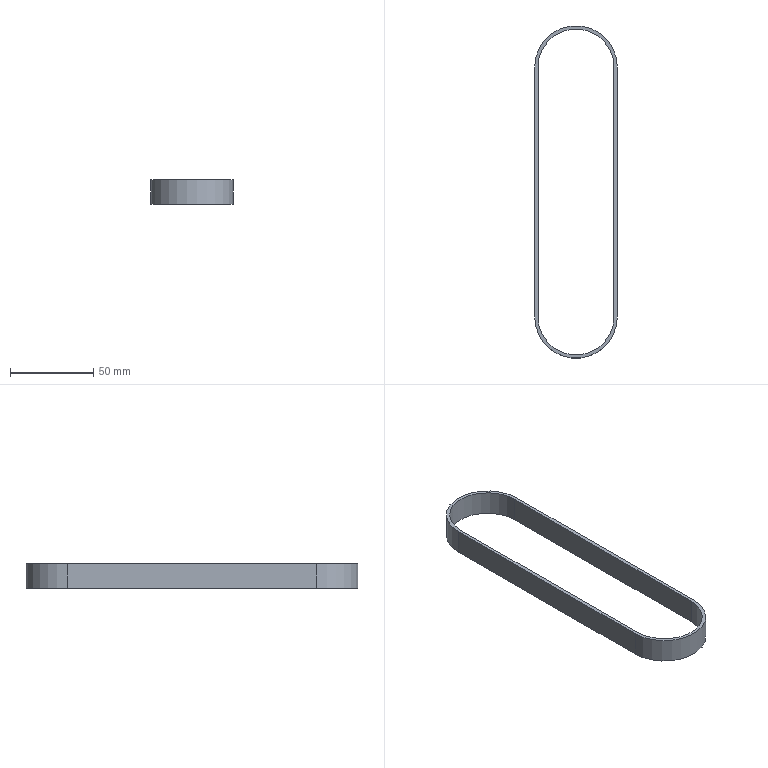Part | STEP file | Belt 1-1^ND25021-刻码机 | 1 solid | 10 faces | box 49.6 x 199.6 x 15 mm | volume 13486 mm3 | plane 6 | cylinder 4 | commonest cylinder face diameters 45.6 x2 49.6 x2
STEP:
#1=CARTESIAN_POINT('',(0.,0.,0.));
#2=DIRECTION('',(0.,0.,1.));
#3=DIRECTION('',(1.,0.,0.));
#4=AXIS2_PLACEMENT_3D('',#1,#2,#3);
#5=CARTESIAN_POINT('',(8.672,136.163,15.));
#6=VERTEX_POINT('',#5);
#7=CARTESIAN_POINT('',(-40.928,136.163,15.));
#8=VERTEX_POINT('',#7);
#9=CARTESIAN_POINT('',(-16.128,136.163,15.));
#10=DIRECTION('',(0.,0.,1.));
#11=DIRECTION('',(-1.,0.,0.));
#12=AXIS2_PLACEMENT_3D('',#9,#10,#11);
#13=CIRCLE('',#12,24.8);
#14=CARTESIAN_POINT('',(-16.128,136.163,15.));
#15=DIRECTION('',(0.,0.,-1.));
#16=DIRECTION('',(-1.,0.,0.));
#17=AXIS2_PLACEMENT_3D('',#14,#15,#16);
#18=PLANE('',#17);
#19=CARTESIAN_POINT('',(24.8,0.));
#20=CARTESIAN_POINT('',(24.8,-42.955));
#21=CARTESIAN_POINT('',(-12.4,-21.477));
#22=CARTESIAN_POINT('',(-49.6,0.));
#23=CARTESIAN_POINT('',(-12.4,21.477));
#24=CARTESIAN_POINT('',(24.8,42.955));
#25=CARTESIAN_POINT('',(24.8,0.));
#26=(BOUNDED_CURVE()B_SPLINE_CURVE(2,(#19,#20,#21,#22,#23,#24,#25),.UNSPECIFIED.,.T.,.F.)B_SPLINE_CURVE_WITH_KNOTS((1,2,2,2,2,1),(-2.094,0.,2.094,4.189,6.283,8.378),.UNSPECIFIED.)CURVE()GEOMETRIC_REPRESENTATION_ITEM()RATIONAL_B_SPLINE_CURVE((1.,0.5,1.,0.5,1.,0.5,1.))REPRESENTATION_ITEM(''));
#27=(GEOMETRIC_REPRESENTATION_CONTEXT(2)PARAMETRIC_REPRESENTATION_CONTEXT()REPRESENTATION_CONTEXT('',''));
#28=DEFINITIONAL_REPRESENTATION('',(#26),#27);
#29=PCURVE('',#18,#28);
#30=CARTESIAN_POINT('',(-16.128,136.163,15.));
#31=DIRECTION('',(0.,0.,-1.));
#32=DIRECTION('',(-1.,0.,0.));
#33=AXIS2_PLACEMENT_3D('',#30,#31,#32);
#34=CYLINDRICAL_SURFACE('',#33,24.8);
#35=CARTESIAN_POINT('',(6.283,0.));
#36=DIRECTION('',(-1.,0.));
#37=VECTOR('',#36,1.);
#38=LINE('',#35,#37);
#39=(GEOMETRIC_REPRESENTATION_CONTEXT(2)PARAMETRIC_REPRESENTATION_CONTEXT()REPRESENTATION_CONTEXT('',''));
#40=DEFINITIONAL_REPRESENTATION('',(#38),#39);
#41=PCURVE('',#34,#40);
#42=SURFACE_CURVE('',#13,(#29,#41),.PCURVE_S1.);
#43=EDGE_CURVE('',#6,#8,#42,.T.);
#44=ORIENTED_EDGE('',*,*,#43,.T.);
#45=CARTESIAN_POINT('',(-40.928,-13.837,15.));
#46=VERTEX_POINT('',#45);
#47=CARTESIAN_POINT('',(-40.928,136.163,15.));
#48=DIRECTION('',(0.,-1.,0.));
#49=VECTOR('',#48,1.);
#50=LINE('',#47,#49);
#51=CARTESIAN_POINT('',(24.8,0.));
#52=DIRECTION('',(0.,-1.));
#53=VECTOR('',#52,1.);
#54=LINE('',#51,#53);
#55=(GEOMETRIC_REPRESENTATION_CONTEXT(2)PARAMETRIC_REPRESENTATION_CONTEXT()REPRESENTATION_CONTEXT('',''));
#56=DEFINITIONAL_REPRESENTATION('',(#54),#55);
#57=PCURVE('',#18,#56);
#58=CARTESIAN_POINT('',(-40.928,136.163,15.));
#59=DIRECTION('',(1.,0.,0.));
#60=DIRECTION('',(0.,0.,-1.));
#61=AXIS2_PLACEMENT_3D('',#58,#59,#60);
#62=PLANE('',#61);
#63=CARTESIAN_POINT('',(0.,0.));
#64=DIRECTION('',(0.,-1.));
#65=VECTOR('',#64,1.);
#66=LINE('',#63,#65);
#67=(GEOMETRIC_REPRESENTATION_CONTEXT(2)PARAMETRIC_REPRESENTATION_CONTEXT()REPRESENTATION_CONTEXT('',''));
#68=DEFINITIONAL_REPRESENTATION('',(#66),#67);
#69=PCURVE('',#62,#68);
#70=SURFACE_CURVE('',#50,(#57,#69),.PCURVE_S1.);
#71=EDGE_CURVE('',#8,#46,#70,.T.);
#72=ORIENTED_EDGE('',*,*,#71,.T.);
#73=CARTESIAN_POINT('',(8.672,-13.837,15.));
#74=VERTEX_POINT('',#73);
#75=CARTESIAN_POINT('',(-16.128,-13.837,15.));
#76=DIRECTION('',(0.,0.,1.));
#77=DIRECTION('',(-1.,0.,0.));
#78=AXIS2_PLACEMENT_3D('',#75,#76,#77);
#79=CIRCLE('',#78,24.8);
#80=CARTESIAN_POINT('',(24.8,-150.));
#81=CARTESIAN_POINT('',(24.8,-192.955));
#82=CARTESIAN_POINT('',(-12.4,-171.477));
#83=CARTESIAN_POINT('',(-49.6,-150.));
#84=CARTESIAN_POINT('',(-12.4,-128.523));
#85=CARTESIAN_POINT('',(24.8,-107.045));
#86=CARTESIAN_POINT('',(24.8,-150.));
#87=(BOUNDED_CURVE()B_SPLINE_CURVE(2,(#80,#81,#82,#83,#84,#85,#86),.UNSPECIFIED.,.T.,.F.)B_SPLINE_CURVE_WITH_KNOTS((1,2,2,2,2,1),(-2.094,0.,2.094,4.189,6.283,8.378),.UNSPECIFIED.)CURVE()GEOMETRIC_REPRESENTATION_ITEM()RATIONAL_B_SPLINE_CURVE((1.,0.5,1.,0.5,1.,0.5,1.))REPRESENTATION_ITEM(''));
#88=(GEOMETRIC_REPRESENTATION_CONTEXT(2)PARAMETRIC_REPRESENTATION_CONTEXT()REPRESENTATION_CONTEXT('',''));
#89=DEFINITIONAL_REPRESENTATION('',(#87),#88);
#90=PCURVE('',#18,#89);
#91=CARTESIAN_POINT('',(-16.128,-13.837,15.));
#92=DIRECTION('',(0.,0.,-1.));
#93=DIRECTION('',(-1.,0.,0.));
#94=AXIS2_PLACEMENT_3D('',#91,#92,#93);
#95=CYLINDRICAL_SURFACE('',#94,24.8);
#96=CARTESIAN_POINT('',(6.283,0.));
#97=DIRECTION('',(-1.,0.));
#98=VECTOR('',#97,1.);
#99=LINE('',#96,#98);
#100=(GEOMETRIC_REPRESENTATION_CONTEXT(2)PARAMETRIC_REPRESENTATION_CONTEXT()REPRESENTATION_CONTEXT('',''));
#101=DEFINITIONAL_REPRESENTATION('',(#99),#100);
#102=PCURVE('',#95,#101);
#103=SURFACE_CURVE('',#79,(#90,#102),.PCURVE_S1.);
#104=EDGE_CURVE('',#46,#74,#103,.T.);
#105=ORIENTED_EDGE('',*,*,#104,.T.);
#106=CARTESIAN_POINT('',(8.672,136.163,15.));
#107=DIRECTION('',(0.,1.,0.));
#108=VECTOR('',#107,1.);
#109=LINE('',#106,#108);
#110=CARTESIAN_POINT('',(-24.8,0.));
#111=DIRECTION('',(0.,1.));
#112=VECTOR('',#111,1.);
#113=LINE('',#110,#112);
#114=(GEOMETRIC_REPRESENTATION_CONTEXT(2)PARAMETRIC_REPRESENTATION_CONTEXT()REPRESENTATION_CONTEXT('',''));
#115=DEFINITIONAL_REPRESENTATION('',(#113),#114);
#116=PCURVE('',#18,#115);
#117=CARTESIAN_POINT('',(8.672,136.163,15.));
#118=DIRECTION('',(-1.,0.,0.));
#119=DIRECTION('',(0.,0.,1.));
#120=AXIS2_PLACEMENT_3D('',#117,#118,#119);
#121=PLANE('',#120);
#122=CARTESIAN_POINT('',(0.,0.));
#123=DIRECTION('',(0.,1.));
#124=VECTOR('',#123,1.);
#125=LINE('',#122,#124);
#126=(GEOMETRIC_REPRESENTATION_CONTEXT(2)PARAMETRIC_REPRESENTATION_CONTEXT()REPRESENTATION_CONTEXT('',''));
#127=DEFINITIONAL_REPRESENTATION('',(#125),#126);
#128=PCURVE('',#121,#127);
#129=SURFACE_CURVE('',#109,(#116,#128),.PCURVE_S1.);
#130=EDGE_CURVE('',#74,#6,#129,.T.);
#131=ORIENTED_EDGE('',*,*,#130,.T.);
#132=EDGE_LOOP('',(#44,#72,#105,#131));
#133=FACE_BOUND('',#132,.T.);
#134=CARTESIAN_POINT('',(6.672,136.163,15.));
#135=VERTEX_POINT('',#134);
#136=CARTESIAN_POINT('',(-38.928,136.163,15.));
#137=VERTEX_POINT('',#136);
#138=CARTESIAN_POINT('',(-16.128,136.163,15.));
#139=DIRECTION('',(0.,0.,1.));
#140=DIRECTION('',(-1.,0.,0.));
#141=AXIS2_PLACEMENT_3D('',#138,#139,#140);
#142=CIRCLE('',#141,22.8);
#143=CARTESIAN_POINT('',(22.8,0.));
#144=CARTESIAN_POINT('',(22.8,-39.491));
#145=CARTESIAN_POINT('',(-11.4,-19.745));
#146=CARTESIAN_POINT('',(-45.6,0.));
#147=CARTESIAN_POINT('',(-11.4,19.745));
#148=CARTESIAN_POINT('',(22.8,39.491));
#149=CARTESIAN_POINT('',(22.8,0.));
#150=(BOUNDED_CURVE()B_SPLINE_CURVE(2,(#143,#144,#145,#146,#147,#148,#149),.UNSPECIFIED.,.T.,.F.)B_SPLINE_CURVE_WITH_KNOTS((1,2,2,2,2,1),(-2.094,0.,2.094,4.189,6.283,8.378),.UNSPECIFIED.)CURVE()GEOMETRIC_REPRESENTATION_ITEM()RATIONAL_B_SPLINE_CURVE((1.,0.5,1.,0.5,1.,0.5,1.))REPRESENTATION_ITEM(''));
#151=(GEOMETRIC_REPRESENTATION_CONTEXT(2)PARAMETRIC_REPRESENTATION_CONTEXT()REPRESENTATION_CONTEXT('',''));
#152=DEFINITIONAL_REPRESENTATION('',(#150),#151);
#153=PCURVE('',#18,#152);
#154=CARTESIAN_POINT('',(-16.128,136.163,15.));
#155=DIRECTION('',(0.,0.,-1.));
#156=DIRECTION('',(-1.,0.,0.));
#157=AXIS2_PLACEMENT_3D('',#154,#155,#156);
#158=CYLINDRICAL_SURFACE('',#157,22.8);
#159=CARTESIAN_POINT('',(6.283,0.));
#160=DIRECTION('',(-1.,0.));
#161=VECTOR('',#160,1.);
#162=LINE('',#159,#161);
#163=(GEOMETRIC_REPRESENTATION_CONTEXT(2)PARAMETRIC_REPRESENTATION_CONTEXT()REPRESENTATION_CONTEXT('',''));
#164=DEFINITIONAL_REPRESENTATION('',(#162),#163);
#165=PCURVE('',#158,#164);
#166=SURFACE_CURVE('',#142,(#153,#165),.PCURVE_S1.);
#167=EDGE_CURVE('',#135,#137,#166,.T.);
#168=ORIENTED_EDGE('',*,*,#167,.F.);
#169=CARTESIAN_POINT('',(6.672,-13.837,15.));
#170=VERTEX_POINT('',#169);
#171=CARTESIAN_POINT('',(6.672,136.163,15.));
#172=DIRECTION('',(0.,1.,0.));
#173=VECTOR('',#172,1.);
#174=LINE('',#171,#173);
#175=CARTESIAN_POINT('',(-22.8,0.));
#176=DIRECTION('',(0.,1.));
#177=VECTOR('',#176,1.);
#178=LINE('',#175,#177);
#179=(GEOMETRIC_REPRESENTATION_CONTEXT(2)PARAMETRIC_REPRESENTATION_CONTEXT()REPRESENTATION_CONTEXT('',''));
#180=DEFINITIONAL_REPRESENTATION('',(#178),#179);
#181=PCURVE('',#18,#180);
#182=CARTESIAN_POINT('',(6.672,136.163,15.));
#183=DIRECTION('',(-1.,0.,0.));
#184=DIRECTION('',(0.,0.,1.));
#185=AXIS2_PLACEMENT_3D('',#182,#183,#184);
#186=PLANE('',#185);
#187=CARTESIAN_POINT('',(0.,0.));
#188=DIRECTION('',(0.,1.));
#189=VECTOR('',#188,1.);
#190=LINE('',#187,#189);
#191=(GEOMETRIC_REPRESENTATION_CONTEXT(2)PARAMETRIC_REPRESENTATION_CONTEXT()REPRESENTATION_CONTEXT('',''));
#192=DEFINITIONAL_REPRESENTATION('',(#190),#191);
#193=PCURVE('',#186,#192);
#194=SURFACE_CURVE('',#174,(#181,#193),.PCURVE_S1.);
#195=EDGE_CURVE('',#170,#135,#194,.T.);
#196=ORIENTED_EDGE('',*,*,#195,.F.);
#197=CARTESIAN_POINT('',(-38.928,-13.837,15.));
#198=VERTEX_POINT('',#197);
#199=CARTESIAN_POINT('',(-16.128,-13.837,15.));
#200=DIRECTION('',(0.,0.,1.));
#201=DIRECTION('',(-1.,0.,0.));
#202=AXIS2_PLACEMENT_3D('',#199,#200,#201);
#203=CIRCLE('',#202,22.8);
#204=CARTESIAN_POINT('',(22.8,-150.));
#205=CARTESIAN_POINT('',(22.8,-189.491));
#206=CARTESIAN_POINT('',(-11.4,-169.745));
#207=CARTESIAN_POINT('',(-45.6,-150.));
#208=CARTESIAN_POINT('',(-11.4,-130.255));
#209=CARTESIAN_POINT('',(22.8,-110.509));
#210=CARTESIAN_POINT('',(22.8,-150.));
#211=(BOUNDED_CURVE()B_SPLINE_CURVE(2,(#204,#205,#206,#207,#208,#209,#210),.UNSPECIFIED.,.T.,.F.)B_SPLINE_CURVE_WITH_KNOTS((1,2,2,2,2,1),(-2.094,0.,2.094,4.189,6.283,8.378),.UNSPECIFIED.)CURVE()GEOMETRIC_REPRESENTATION_ITEM()RATIONAL_B_SPLINE_CURVE((1.,0.5,1.,0.5,1.,0.5,1.))REPRESENTATION_ITEM(''));
#212=(GEOMETRIC_REPRESENTATION_CONTEXT(2)PARAMETRIC_REPRESENTATION_CONTEXT()REPRESENTATION_CONTEXT('',''));
#213=DEFINITIONAL_REPRESENTATION('',(#211),#212);
#214=PCURVE('',#18,#213);
#215=CARTESIAN_POINT('',(-16.128,-13.837,15.));
#216=DIRECTION('',(0.,0.,-1.));
#217=DIRECTION('',(-1.,0.,0.));
#218=AXIS2_PLACEMENT_3D('',#215,#216,#217);
#219=CYLINDRICAL_SURFACE('',#218,22.8);
#220=CARTESIAN_POINT('',(6.283,0.));
#221=DIRECTION('',(-1.,0.));
#222=VECTOR('',#221,1.);
#223=LINE('',#220,#222);
#224=(GEOMETRIC_REPRESENTATION_CONTEXT(2)PARAMETRIC_REPRESENTATION_CONTEXT()REPRESENTATION_CONTEXT('',''));
#225=DEFINITIONAL_REPRESENTATION('',(#223),#224);
#226=PCURVE('',#219,#225);
#227=SURFACE_CURVE('',#203,(#214,#226),.PCURVE_S1.);
#228=EDGE_CURVE('',#198,#170,#227,.T.);
#229=ORIENTED_EDGE('',*,*,#228,.F.);
#230=CARTESIAN_POINT('',(-38.928,-13.837,15.));
#231=DIRECTION('',(0.,-1.,0.));
#232=VECTOR('',#231,1.);
#233=LINE('',#230,#232);
#234=CARTESIAN_POINT('',(22.8,-150.));
#235=DIRECTION('',(0.,-1.));
#236=VECTOR('',#235,1.);
#237=LINE('',#234,#236);
#238=(GEOMETRIC_REPRESENTATION_CONTEXT(2)PARAMETRIC_REPRESENTATION_CONTEXT()REPRESENTATION_CONTEXT('',''));
#239=DEFINITIONAL_REPRESENTATION('',(#237),#238);
#240=PCURVE('',#18,#239);
#241=CARTESIAN_POINT('',(-38.928,-13.837,15.));
#242=DIRECTION('',(1.,0.,0.));
#243=DIRECTION('',(0.,0.,-1.));
#244=AXIS2_PLACEMENT_3D('',#241,#242,#243);
#245=PLANE('',#244);
#246=CARTESIAN_POINT('',(0.,0.));
#247=DIRECTION('',(0.,-1.));
#248=VECTOR('',#247,1.);
#249=LINE('',#246,#248);
#250=(GEOMETRIC_REPRESENTATION_CONTEXT(2)PARAMETRIC_REPRESENTATION_CONTEXT()REPRESENTATION_CONTEXT('',''));
#251=DEFINITIONAL_REPRESENTATION('',(#249),#250);
#252=PCURVE('',#245,#251);
#253=SURFACE_CURVE('',#233,(#240,#252),.PCURVE_S1.);
#254=EDGE_CURVE('',#137,#198,#253,.T.);
#255=ORIENTED_EDGE('',*,*,#254,.F.);
#256=EDGE_LOOP('',(#168,#196,#229,#255));
#257=FACE_BOUND('',#256,.T.);
#258=ADVANCED_FACE('',(#133,#257),#18,.F.);
#259=CARTESIAN_POINT('',(8.672,136.163,0.));
#260=VERTEX_POINT('',#259);
#261=CARTESIAN_POINT('',(-40.928,136.163,0.));
#262=VERTEX_POINT('',#261);
#263=CARTESIAN_POINT('',(-16.128,136.163,0.));
#264=DIRECTION('',(0.,0.,1.));
#265=DIRECTION('',(-1.,0.,0.));
#266=AXIS2_PLACEMENT_3D('',#263,#264,#265);
#267=CIRCLE('',#266,24.8);
#268=CARTESIAN_POINT('',(-16.128,136.163,0.));
#269=DIRECTION('',(0.,0.,-1.));
#270=DIRECTION('',(-1.,0.,0.));
#271=AXIS2_PLACEMENT_3D('',#268,#269,#270);
#272=PLANE('',#271);
#273=CARTESIAN_POINT('',(24.8,0.));
#274=CARTESIAN_POINT('',(24.8,-42.955));
#275=CARTESIAN_POINT('',(-12.4,-21.477));
#276=CARTESIAN_POINT('',(-49.6,0.));
#277=CARTESIAN_POINT('',(-12.4,21.477));
#278=CARTESIAN_POINT('',(24.8,42.955));
#279=CARTESIAN_POINT('',(24.8,0.));
#280=(BOUNDED_CURVE()B_SPLINE_CURVE(2,(#273,#274,#275,#276,#277,#278,#279),.UNSPECIFIED.,.T.,.F.)B_SPLINE_CURVE_WITH_KNOTS((1,2,2,2,2,1),(-2.094,0.,2.094,4.189,6.283,8.378),.UNSPECIFIED.)CURVE()GEOMETRIC_REPRESENTATION_ITEM()RATIONAL_B_SPLINE_CURVE((1.,0.5,1.,0.5,1.,0.5,1.))REPRESENTATION_ITEM(''));
#281=(GEOMETRIC_REPRESENTATION_CONTEXT(2)PARAMETRIC_REPRESENTATION_CONTEXT()REPRESENTATION_CONTEXT('',''));
#282=DEFINITIONAL_REPRESENTATION('',(#280),#281);
#283=PCURVE('',#272,#282);
#284=CARTESIAN_POINT('',(6.283,15.));
#285=DIRECTION('',(-1.,0.));
#286=VECTOR('',#285,1.);
#287=LINE('',#284,#286);
#288=(GEOMETRIC_REPRESENTATION_CONTEXT(2)PARAMETRIC_REPRESENTATION_CONTEXT()REPRESENTATION_CONTEXT('',''));
#289=DEFINITIONAL_REPRESENTATION('',(#287),#288);
#290=PCURVE('',#34,#289);
#291=SURFACE_CURVE('',#267,(#283,#290),.PCURVE_S1.);
#292=EDGE_CURVE('',#260,#262,#291,.T.);
#293=ORIENTED_EDGE('',*,*,#292,.F.);
#294=CARTESIAN_POINT('',(8.672,-13.837,0.));
#295=VERTEX_POINT('',#294);
#296=CARTESIAN_POINT('',(8.672,136.163,0.));
#297=DIRECTION('',(0.,1.,0.));
#298=VECTOR('',#297,1.);
#299=LINE('',#296,#298);
#300=CARTESIAN_POINT('',(-24.8,0.));
#301=DIRECTION('',(0.,1.));
#302=VECTOR('',#301,1.);
#303=LINE('',#300,#302);
#304=(GEOMETRIC_REPRESENTATION_CONTEXT(2)PARAMETRIC_REPRESENTATION_CONTEXT()REPRESENTATION_CONTEXT('',''));
#305=DEFINITIONAL_REPRESENTATION('',(#303),#304);
#306=PCURVE('',#272,#305);
#307=CARTESIAN_POINT('',(-15.,0.));
#308=DIRECTION('',(0.,1.));
#309=VECTOR('',#308,1.);
#310=LINE('',#307,#309);
#311=(GEOMETRIC_REPRESENTATION_CONTEXT(2)PARAMETRIC_REPRESENTATION_CONTEXT()REPRESENTATION_CONTEXT('',''));
#312=DEFINITIONAL_REPRESENTATION('',(#310),#311);
#313=PCURVE('',#121,#312);
#314=SURFACE_CURVE('',#299,(#306,#313),.PCURVE_S1.);
#315=EDGE_CURVE('',#295,#260,#314,.T.);
#316=ORIENTED_EDGE('',*,*,#315,.F.);
#317=CARTESIAN_POINT('',(-40.928,-13.837,0.));
#318=VERTEX_POINT('',#317);
#319=CARTESIAN_POINT('',(-16.128,-13.837,0.));
#320=DIRECTION('',(0.,0.,1.));
#321=DIRECTION('',(-1.,0.,0.));
#322=AXIS2_PLACEMENT_3D('',#319,#320,#321);
#323=CIRCLE('',#322,24.8);
#324=CARTESIAN_POINT('',(24.8,-150.));
#325=CARTESIAN_POINT('',(24.8,-192.955));
#326=CARTESIAN_POINT('',(-12.4,-171.477));
#327=CARTESIAN_POINT('',(-49.6,-150.));
#328=CARTESIAN_POINT('',(-12.4,-128.523));
#329=CARTESIAN_POINT('',(24.8,-107.045));
#330=CARTESIAN_POINT('',(24.8,-150.));
#331=(BOUNDED_CURVE()B_SPLINE_CURVE(2,(#324,#325,#326,#327,#328,#329,#330),.UNSPECIFIED.,.T.,.F.)B_SPLINE_CURVE_WITH_KNOTS((1,2,2,2,2,1),(-2.094,0.,2.094,4.189,6.283,8.378),.UNSPECIFIED.)CURVE()GEOMETRIC_REPRESENTATION_ITEM()RATIONAL_B_SPLINE_CURVE((1.,0.5,1.,0.5,1.,0.5,1.))REPRESENTATION_ITEM(''));
#332=(GEOMETRIC_REPRESENTATION_CONTEXT(2)PARAMETRIC_REPRESENTATION_CONTEXT()REPRESENTATION_CONTEXT('',''));
#333=DEFINITIONAL_REPRESENTATION('',(#331),#332);
#334=PCURVE('',#272,#333);
#335=CARTESIAN_POINT('',(6.283,15.));
#336=DIRECTION('',(-1.,0.));
#337=VECTOR('',#336,1.);
#338=LINE('',#335,#337);
#339=(GEOMETRIC_REPRESENTATION_CONTEXT(2)PARAMETRIC_REPRESENTATION_CONTEXT()REPRESENTATION_CONTEXT('',''));
#340=DEFINITIONAL_REPRESENTATION('',(#338),#339);
#341=PCURVE('',#95,#340);
#342=SURFACE_CURVE('',#323,(#334,#341),.PCURVE_S1.);
#343=EDGE_CURVE('',#318,#295,#342,.T.);
#344=ORIENTED_EDGE('',*,*,#343,.F.);
#345=CARTESIAN_POINT('',(-40.928,136.163,0.));
#346=DIRECTION('',(0.,-1.,0.));
#347=VECTOR('',#346,1.);
#348=LINE('',#345,#347);
#349=CARTESIAN_POINT('',(24.8,0.));
#350=DIRECTION('',(0.,-1.));
#351=VECTOR('',#350,1.);
#352=LINE('',#349,#351);
#353=(GEOMETRIC_REPRESENTATION_CONTEXT(2)PARAMETRIC_REPRESENTATION_CONTEXT()REPRESENTATION_CONTEXT('',''));
#354=DEFINITIONAL_REPRESENTATION('',(#352),#353);
#355=PCURVE('',#272,#354);
#356=CARTESIAN_POINT('',(15.,0.));
#357=DIRECTION('',(0.,-1.));
#358=VECTOR('',#357,1.);
#359=LINE('',#356,#358);
#360=(GEOMETRIC_REPRESENTATION_CONTEXT(2)PARAMETRIC_REPRESENTATION_CONTEXT()REPRESENTATION_CONTEXT('',''));
#361=DEFINITIONAL_REPRESENTATION('',(#359),#360);
#362=PCURVE('',#62,#361);
#363=SURFACE_CURVE('',#348,(#355,#362),.PCURVE_S1.);
#364=EDGE_CURVE('',#262,#318,#363,.T.);
#365=ORIENTED_EDGE('',*,*,#364,.F.);
#366=EDGE_LOOP('',(#293,#316,#344,#365));
#367=FACE_BOUND('',#366,.T.);
#368=CARTESIAN_POINT('',(6.672,-13.837,0.));
#369=VERTEX_POINT('',#368);
#370=CARTESIAN_POINT('',(6.672,136.163,0.));
#371=VERTEX_POINT('',#370);
#372=CARTESIAN_POINT('',(6.672,136.163,0.));
#373=DIRECTION('',(0.,1.,0.));
#374=VECTOR('',#373,1.);
#375=LINE('',#372,#374);
#376=CARTESIAN_POINT('',(-22.8,0.));
#377=DIRECTION('',(0.,1.));
#378=VECTOR('',#377,1.);
#379=LINE('',#376,#378);
#380=(GEOMETRIC_REPRESENTATION_CONTEXT(2)PARAMETRIC_REPRESENTATION_CONTEXT()REPRESENTATION_CONTEXT('',''));
#381=DEFINITIONAL_REPRESENTATION('',(#379),#380);
#382=PCURVE('',#272,#381);
#383=CARTESIAN_POINT('',(-15.,0.));
#384=DIRECTION('',(0.,1.));
#385=VECTOR('',#384,1.);
#386=LINE('',#383,#385);
#387=(GEOMETRIC_REPRESENTATION_CONTEXT(2)PARAMETRIC_REPRESENTATION_CONTEXT()REPRESENTATION_CONTEXT('',''));
#388=DEFINITIONAL_REPRESENTATION('',(#386),#387);
#389=PCURVE('',#186,#388);
#390=SURFACE_CURVE('',#375,(#382,#389),.PCURVE_S1.);
#391=EDGE_CURVE('',#369,#371,#390,.T.);
#392=ORIENTED_EDGE('',*,*,#391,.T.);
#393=CARTESIAN_POINT('',(-38.928,136.163,0.));
#394=VERTEX_POINT('',#393);
#395=CARTESIAN_POINT('',(-16.128,136.163,0.));
#396=DIRECTION('',(0.,0.,1.));
#397=DIRECTION('',(-1.,0.,0.));
#398=AXIS2_PLACEMENT_3D('',#395,#396,#397);
#399=CIRCLE('',#398,22.8);
#400=CARTESIAN_POINT('',(22.8,0.));
#401=CARTESIAN_POINT('',(22.8,-39.491));
#402=CARTESIAN_POINT('',(-11.4,-19.745));
#403=CARTESIAN_POINT('',(-45.6,0.));
#404=CARTESIAN_POINT('',(-11.4,19.745));
#405=CARTESIAN_POINT('',(22.8,39.491));
#406=CARTESIAN_POINT('',(22.8,0.));
#407=(BOUNDED_CURVE()B_SPLINE_CURVE(2,(#400,#401,#402,#403,#404,#405,#406),.UNSPECIFIED.,.T.,.F.)B_SPLINE_CURVE_WITH_KNOTS((1,2,2,2,2,1),(-2.094,0.,2.094,4.189,6.283,8.378),.UNSPECIFIED.)CURVE()GEOMETRIC_REPRESENTATION_ITEM()RATIONAL_B_SPLINE_CURVE((1.,0.5,1.,0.5,1.,0.5,1.))REPRESENTATION_ITEM(''));
#408=(GEOMETRIC_REPRESENTATION_CONTEXT(2)PARAMETRIC_REPRESENTATION_CONTEXT()REPRESENTATION_CONTEXT('',''));
#409=DEFINITIONAL_REPRESENTATION('',(#407),#408);
#410=PCURVE('',#272,#409);
#411=CARTESIAN_POINT('',(6.283,15.));
#412=DIRECTION('',(-1.,0.));
#413=VECTOR('',#412,1.);
#414=LINE('',#411,#413);
#415=(GEOMETRIC_REPRESENTATION_CONTEXT(2)PARAMETRIC_REPRESENTATION_CONTEXT()REPRESENTATION_CONTEXT('',''));
#416=DEFINITIONAL_REPRESENTATION('',(#414),#415);
#417=PCURVE('',#158,#416);
#418=SURFACE_CURVE('',#399,(#410,#417),.PCURVE_S1.);
#419=EDGE_CURVE('',#371,#394,#418,.T.);
#420=ORIENTED_EDGE('',*,*,#419,.T.);
#421=CARTESIAN_POINT('',(-38.928,-13.837,0.));
#422=VERTEX_POINT('',#421);
#423=CARTESIAN_POINT('',(-38.928,-13.837,0.));
#424=DIRECTION('',(0.,-1.,0.));
#425=VECTOR('',#424,1.);
#426=LINE('',#423,#425);
#427=CARTESIAN_POINT('',(22.8,-150.));
#428=DIRECTION('',(0.,-1.));
#429=VECTOR('',#428,1.);
#430=LINE('',#427,#429);
#431=(GEOMETRIC_REPRESENTATION_CONTEXT(2)PARAMETRIC_REPRESENTATION_CONTEXT()REPRESENTATION_CONTEXT('',''));
#432=DEFINITIONAL_REPRESENTATION('',(#430),#431);
#433=PCURVE('',#272,#432);
#434=CARTESIAN_POINT('',(15.,0.));
#435=DIRECTION('',(0.,-1.));
#436=VECTOR('',#435,1.);
#437=LINE('',#434,#436);
#438=(GEOMETRIC_REPRESENTATION_CONTEXT(2)PARAMETRIC_REPRESENTATION_CONTEXT()REPRESENTATION_CONTEXT('',''));
#439=DEFINITIONAL_REPRESENTATION('',(#437),#438);
#440=PCURVE('',#245,#439);
#441=SURFACE_CURVE('',#426,(#433,#440),.PCURVE_S1.);
#442=EDGE_CURVE('',#394,#422,#441,.T.);
#443=ORIENTED_EDGE('',*,*,#442,.T.);
#444=CARTESIAN_POINT('',(-16.128,-13.837,0.));
#445=DIRECTION('',(0.,0.,1.));
#446=DIRECTION('',(-1.,0.,0.));
#447=AXIS2_PLACEMENT_3D('',#444,#445,#446);
#448=CIRCLE('',#447,22.8);
#449=CARTESIAN_POINT('',(22.8,-150.));
#450=CARTESIAN_POINT('',(22.8,-189.491));
#451=CARTESIAN_POINT('',(-11.4,-169.745));
#452=CARTESIAN_POINT('',(-45.6,-150.));
#453=CARTESIAN_POINT('',(-11.4,-130.255));
#454=CARTESIAN_POINT('',(22.8,-110.509));
#455=CARTESIAN_POINT('',(22.8,-150.));
#456=(BOUNDED_CURVE()B_SPLINE_CURVE(2,(#449,#450,#451,#452,#453,#454,#455),.UNSPECIFIED.,.T.,.F.)B_SPLINE_CURVE_WITH_KNOTS((1,2,2,2,2,1),(-2.094,0.,2.094,4.189,6.283,8.378),.UNSPECIFIED.)CURVE()GEOMETRIC_REPRESENTATION_ITEM()RATIONAL_B_SPLINE_CURVE((1.,0.5,1.,0.5,1.,0.5,1.))REPRESENTATION_ITEM(''));
#457=(GEOMETRIC_REPRESENTATION_CONTEXT(2)PARAMETRIC_REPRESENTATION_CONTEXT()REPRESENTATION_CONTEXT('',''));
#458=DEFINITIONAL_REPRESENTATION('',(#456),#457);
#459=PCURVE('',#272,#458);
#460=CARTESIAN_POINT('',(6.283,15.));
#461=DIRECTION('',(-1.,0.));
#462=VECTOR('',#461,1.);
#463=LINE('',#460,#462);
#464=(GEOMETRIC_REPRESENTATION_CONTEXT(2)PARAMETRIC_REPRESENTATION_CONTEXT()REPRESENTATION_CONTEXT('',''));
#465=DEFINITIONAL_REPRESENTATION('',(#463),#464);
#466=PCURVE('',#219,#465);
#467=SURFACE_CURVE('',#448,(#459,#466),.PCURVE_S1.);
#468=EDGE_CURVE('',#422,#369,#467,.T.);
#469=ORIENTED_EDGE('',*,*,#468,.T.);
#470=EDGE_LOOP('',(#392,#420,#443,#469));
#471=FACE_BOUND('',#470,.T.);
#472=ADVANCED_FACE('',(#367,#471),#272,.T.);
#473=ORIENTED_EDGE('',*,*,#292,.T.);
#474=CARTESIAN_POINT('',(-40.928,136.163,15.));
#475=DIRECTION('',(0.,0.,-1.));
#476=VECTOR('',#475,1.);
#477=LINE('',#474,#476);
#478=CARTESIAN_POINT('',(0.,0.));
#479=DIRECTION('',(0.,1.));
#480=VECTOR('',#479,1.);
#481=LINE('',#478,#480);
#482=(GEOMETRIC_REPRESENTATION_CONTEXT(2)PARAMETRIC_REPRESENTATION_CONTEXT()REPRESENTATION_CONTEXT('',''));
#483=DEFINITIONAL_REPRESENTATION('',(#481),#482);
#484=PCURVE('',#34,#483);
#485=CARTESIAN_POINT('',(0.,0.));
#486=DIRECTION('',(1.,0.));
#487=VECTOR('',#486,1.);
#488=LINE('',#485,#487);
#489=(GEOMETRIC_REPRESENTATION_CONTEXT(2)PARAMETRIC_REPRESENTATION_CONTEXT()REPRESENTATION_CONTEXT('',''));
#490=DEFINITIONAL_REPRESENTATION('',(#488),#489);
#491=PCURVE('',#62,#490);
#492=SURFACE_CURVE('',#477,(#484,#491),.PCURVE_S1.);
#493=EDGE_CURVE('',#8,#262,#492,.T.);
#494=ORIENTED_EDGE('',*,*,#493,.F.);
#495=ORIENTED_EDGE('',*,*,#43,.F.);
#496=CARTESIAN_POINT('',(8.672,136.163,15.));
#497=DIRECTION('',(0.,0.,-1.));
#498=VECTOR('',#497,1.);
#499=LINE('',#496,#498);
#500=CARTESIAN_POINT('',(3.142,0.));
#501=DIRECTION('',(0.,1.));
#502=VECTOR('',#501,1.);
#503=LINE('',#500,#502);
#504=(GEOMETRIC_REPRESENTATION_CONTEXT(2)PARAMETRIC_REPRESENTATION_CONTEXT()REPRESENTATION_CONTEXT('',''));
#505=DEFINITIONAL_REPRESENTATION('',(#503),#504);
#506=PCURVE('',#34,#505);
#507=CARTESIAN_POINT('',(0.,0.));
#508=DIRECTION('',(-1.,0.));
#509=VECTOR('',#508,1.);
#510=LINE('',#507,#509);
#511=(GEOMETRIC_REPRESENTATION_CONTEXT(2)PARAMETRIC_REPRESENTATION_CONTEXT()REPRESENTATION_CONTEXT('',''));
#512=DEFINITIONAL_REPRESENTATION('',(#510),#511);
#513=PCURVE('',#121,#512);
#514=SURFACE_CURVE('',#499,(#506,#513),.PCURVE_S1.);
#515=EDGE_CURVE('',#6,#260,#514,.T.);
#516=ORIENTED_EDGE('',*,*,#515,.T.);
#517=EDGE_LOOP('',(#473,#494,#495,#516));
#518=FACE_BOUND('',#517,.T.);
#519=ADVANCED_FACE('',(#518),#34,.T.);
#520=ORIENTED_EDGE('',*,*,#364,.T.);
#521=CARTESIAN_POINT('',(-40.928,-13.837,15.));
#522=DIRECTION('',(0.,0.,-1.));
#523=VECTOR('',#522,1.);
#524=LINE('',#521,#523);
#525=CARTESIAN_POINT('',(0.,-150.));
#526=DIRECTION('',(1.,0.));
#527=VECTOR('',#526,1.);
#528=LINE('',#525,#527);
#529=(GEOMETRIC_REPRESENTATION_CONTEXT(2)PARAMETRIC_REPRESENTATION_CONTEXT()REPRESENTATION_CONTEXT('',''));
#530=DEFINITIONAL_REPRESENTATION('',(#528),#529);
#531=PCURVE('',#62,#530);
#532=CARTESIAN_POINT('',(6.283,0.));
#533=DIRECTION('',(0.,1.));
#534=VECTOR('',#533,1.);
#535=LINE('',#532,#534);
#536=(GEOMETRIC_REPRESENTATION_CONTEXT(2)PARAMETRIC_REPRESENTATION_CONTEXT()REPRESENTATION_CONTEXT('',''));
#537=DEFINITIONAL_REPRESENTATION('',(#535),#536);
#538=PCURVE('',#95,#537);
#539=SURFACE_CURVE('',#524,(#531,#538),.PCURVE_S1.);
#540=EDGE_CURVE('',#46,#318,#539,.T.);
#541=ORIENTED_EDGE('',*,*,#540,.F.);
#542=ORIENTED_EDGE('',*,*,#71,.F.);
#543=ORIENTED_EDGE('',*,*,#493,.T.);
#544=EDGE_LOOP('',(#520,#541,#542,#543));
#545=FACE_BOUND('',#544,.T.);
#546=ADVANCED_FACE('',(#545),#62,.F.);
#547=ORIENTED_EDGE('',*,*,#343,.T.);
#548=CARTESIAN_POINT('',(8.672,-13.837,15.));
#549=DIRECTION('',(0.,0.,-1.));
#550=VECTOR('',#549,1.);
#551=LINE('',#548,#550);
#552=CARTESIAN_POINT('',(3.142,0.));
#553=DIRECTION('',(0.,1.));
#554=VECTOR('',#553,1.);
#555=LINE('',#552,#554);
#556=(GEOMETRIC_REPRESENTATION_CONTEXT(2)PARAMETRIC_REPRESENTATION_CONTEXT()REPRESENTATION_CONTEXT('',''));
#557=DEFINITIONAL_REPRESENTATION('',(#555),#556);
#558=PCURVE('',#95,#557);
#559=CARTESIAN_POINT('',(0.,-150.));
#560=DIRECTION('',(-1.,0.));
#561=VECTOR('',#560,1.);
#562=LINE('',#559,#561);
#563=(GEOMETRIC_REPRESENTATION_CONTEXT(2)PARAMETRIC_REPRESENTATION_CONTEXT()REPRESENTATION_CONTEXT('',''));
#564=DEFINITIONAL_REPRESENTATION('',(#562),#563);
#565=PCURVE('',#121,#564);
#566=SURFACE_CURVE('',#551,(#558,#565),.PCURVE_S1.);
#567=EDGE_CURVE('',#74,#295,#566,.T.);
#568=ORIENTED_EDGE('',*,*,#567,.F.);
#569=ORIENTED_EDGE('',*,*,#104,.F.);
#570=ORIENTED_EDGE('',*,*,#540,.T.);
#571=EDGE_LOOP('',(#547,#568,#569,#570));
#572=FACE_BOUND('',#571,.T.);
#573=ADVANCED_FACE('',(#572),#95,.T.);
#574=ORIENTED_EDGE('',*,*,#315,.T.);
#575=ORIENTED_EDGE('',*,*,#515,.F.);
#576=ORIENTED_EDGE('',*,*,#130,.F.);
#577=ORIENTED_EDGE('',*,*,#567,.T.);
#578=EDGE_LOOP('',(#574,#575,#576,#577));
#579=FACE_BOUND('',#578,.T.);
#580=ADVANCED_FACE('',(#579),#121,.F.);
#581=CARTESIAN_POINT('',(-38.928,136.163,15.));
#582=DIRECTION('',(0.,0.,-1.));
#583=VECTOR('',#582,1.);
#584=LINE('',#581,#583);
#585=CARTESIAN_POINT('',(0.,0.));
#586=DIRECTION('',(0.,1.));
#587=VECTOR('',#586,1.);
#588=LINE('',#585,#587);
#589=(GEOMETRIC_REPRESENTATION_CONTEXT(2)PARAMETRIC_REPRESENTATION_CONTEXT()REPRESENTATION_CONTEXT('',''));
#590=DEFINITIONAL_REPRESENTATION('',(#588),#589);
#591=PCURVE('',#158,#590);
#592=CARTESIAN_POINT('',(0.,150.));
#593=DIRECTION('',(1.,0.));
#594=VECTOR('',#593,1.);
#595=LINE('',#592,#594);
#596=(GEOMETRIC_REPRESENTATION_CONTEXT(2)PARAMETRIC_REPRESENTATION_CONTEXT()REPRESENTATION_CONTEXT('',''));
#597=DEFINITIONAL_REPRESENTATION('',(#595),#596);
#598=PCURVE('',#245,#597);
#599=SURFACE_CURVE('',#584,(#591,#598),.PCURVE_S1.);
#600=EDGE_CURVE('',#137,#394,#599,.T.);
#601=ORIENTED_EDGE('',*,*,#600,.F.);
#602=ORIENTED_EDGE('',*,*,#167,.F.);
#603=CARTESIAN_POINT('',(6.672,136.163,15.));
#604=DIRECTION('',(0.,0.,-1.));
#605=VECTOR('',#604,1.);
#606=LINE('',#603,#605);
#607=CARTESIAN_POINT('',(3.142,0.));
#608=DIRECTION('',(0.,1.));
#609=VECTOR('',#608,1.);
#610=LINE('',#607,#609);
#611=(GEOMETRIC_REPRESENTATION_CONTEXT(2)PARAMETRIC_REPRESENTATION_CONTEXT()REPRESENTATION_CONTEXT('',''));
#612=DEFINITIONAL_REPRESENTATION('',(#610),#611);
#613=PCURVE('',#158,#612);
#614=CARTESIAN_POINT('',(0.,0.));
#615=DIRECTION('',(-1.,0.));
#616=VECTOR('',#615,1.);
#617=LINE('',#614,#616);
#618=(GEOMETRIC_REPRESENTATION_CONTEXT(2)PARAMETRIC_REPRESENTATION_CONTEXT()REPRESENTATION_CONTEXT('',''));
#619=DEFINITIONAL_REPRESENTATION('',(#617),#618);
#620=PCURVE('',#186,#619);
#621=SURFACE_CURVE('',#606,(#613,#620),.PCURVE_S1.);
#622=EDGE_CURVE('',#135,#371,#621,.T.);
#623=ORIENTED_EDGE('',*,*,#622,.T.);
#624=ORIENTED_EDGE('',*,*,#419,.T.);
#625=EDGE_LOOP('',(#601,#602,#623,#624));
#626=FACE_BOUND('',#625,.F.);
#627=ADVANCED_FACE('',(#626),#158,.F.);
#628=ORIENTED_EDGE('',*,*,#442,.F.);
#629=ORIENTED_EDGE('',*,*,#600,.F.);
#630=ORIENTED_EDGE('',*,*,#254,.T.);
#631=CARTESIAN_POINT('',(-38.928,-13.837,15.));
#632=DIRECTION('',(0.,0.,-1.));
#633=VECTOR('',#632,1.);
#634=LINE('',#631,#633);
#635=CARTESIAN_POINT('',(0.,0.));
#636=DIRECTION('',(1.,0.));
#637=VECTOR('',#636,1.);
#638=LINE('',#635,#637);
#639=(GEOMETRIC_REPRESENTATION_CONTEXT(2)PARAMETRIC_REPRESENTATION_CONTEXT()REPRESENTATION_CONTEXT('',''));
#640=DEFINITIONAL_REPRESENTATION('',(#638),#639);
#641=PCURVE('',#245,#640);
#642=CARTESIAN_POINT('',(6.283,0.));
#643=DIRECTION('',(0.,1.));
#644=VECTOR('',#643,1.);
#645=LINE('',#642,#644);
#646=(GEOMETRIC_REPRESENTATION_CONTEXT(2)PARAMETRIC_REPRESENTATION_CONTEXT()REPRESENTATION_CONTEXT('',''));
#647=DEFINITIONAL_REPRESENTATION('',(#645),#646);
#648=PCURVE('',#219,#647);
#649=SURFACE_CURVE('',#634,(#641,#648),.PCURVE_S1.);
#650=EDGE_CURVE('',#198,#422,#649,.T.);
#651=ORIENTED_EDGE('',*,*,#650,.T.);
#652=EDGE_LOOP('',(#628,#629,#630,#651));
#653=FACE_BOUND('',#652,.T.);
#654=ADVANCED_FACE('',(#653),#245,.T.);
#655=CARTESIAN_POINT('',(6.672,-13.837,15.));
#656=DIRECTION('',(0.,0.,-1.));
#657=VECTOR('',#656,1.);
#658=LINE('',#655,#657);
#659=CARTESIAN_POINT('',(3.142,0.));
#660=DIRECTION('',(0.,1.));
#661=VECTOR('',#660,1.);
#662=LINE('',#659,#661);
#663=(GEOMETRIC_REPRESENTATION_CONTEXT(2)PARAMETRIC_REPRESENTATION_CONTEXT()REPRESENTATION_CONTEXT('',''));
#664=DEFINITIONAL_REPRESENTATION('',(#662),#663);
#665=PCURVE('',#219,#664);
#666=CARTESIAN_POINT('',(0.,-150.));
#667=DIRECTION('',(-1.,0.));
#668=VECTOR('',#667,1.);
#669=LINE('',#666,#668);
#670=(GEOMETRIC_REPRESENTATION_CONTEXT(2)PARAMETRIC_REPRESENTATION_CONTEXT()REPRESENTATION_CONTEXT('',''));
#671=DEFINITIONAL_REPRESENTATION('',(#669),#670);
#672=PCURVE('',#186,#671);
#673=SURFACE_CURVE('',#658,(#665,#672),.PCURVE_S1.);
#674=EDGE_CURVE('',#170,#369,#673,.T.);
#675=ORIENTED_EDGE('',*,*,#674,.F.);
#676=ORIENTED_EDGE('',*,*,#228,.F.);
#677=ORIENTED_EDGE('',*,*,#650,.T.);
#678=ORIENTED_EDGE('',*,*,#468,.T.);
#679=EDGE_LOOP('',(#675,#676,#677,#678));
#680=FACE_BOUND('',#679,.F.);
#681=ADVANCED_FACE('',(#680),#219,.F.);
#682=ORIENTED_EDGE('',*,*,#391,.F.);
#683=ORIENTED_EDGE('',*,*,#674,.F.);
#684=ORIENTED_EDGE('',*,*,#195,.T.);
#685=ORIENTED_EDGE('',*,*,#622,.T.);
#686=EDGE_LOOP('',(#682,#683,#684,#685));
#687=FACE_BOUND('',#686,.T.);
#688=ADVANCED_FACE('',(#687),#186,.T.);
#689=CLOSED_SHELL('',(#258,#472,#519,#546,#573,#580,#627,#654,#681,#688));
#690=MANIFOLD_SOLID_BREP('',#689);
#691=(LENGTH_UNIT()NAMED_UNIT(*)SI_UNIT(.MILLI.,.METRE.));
#692=UNCERTAINTY_MEASURE_WITH_UNIT(LENGTH_MEASURE(0.0000001),#691,'','');
#693=(NAMED_UNIT(*)PLANE_ANGLE_UNIT()SI_UNIT($,.RADIAN.));
#694=(NAMED_UNIT(*)SI_UNIT($,.STERADIAN.)SOLID_ANGLE_UNIT());
#695=(GEOMETRIC_REPRESENTATION_CONTEXT(3)GLOBAL_UNCERTAINTY_ASSIGNED_CONTEXT((#692))GLOBAL_UNIT_ASSIGNED_CONTEXT((#691,#693,#694))REPRESENTATION_CONTEXT('',''));
#696=ADVANCED_BREP_SHAPE_REPRESENTATION('',(#4,#690),#695);